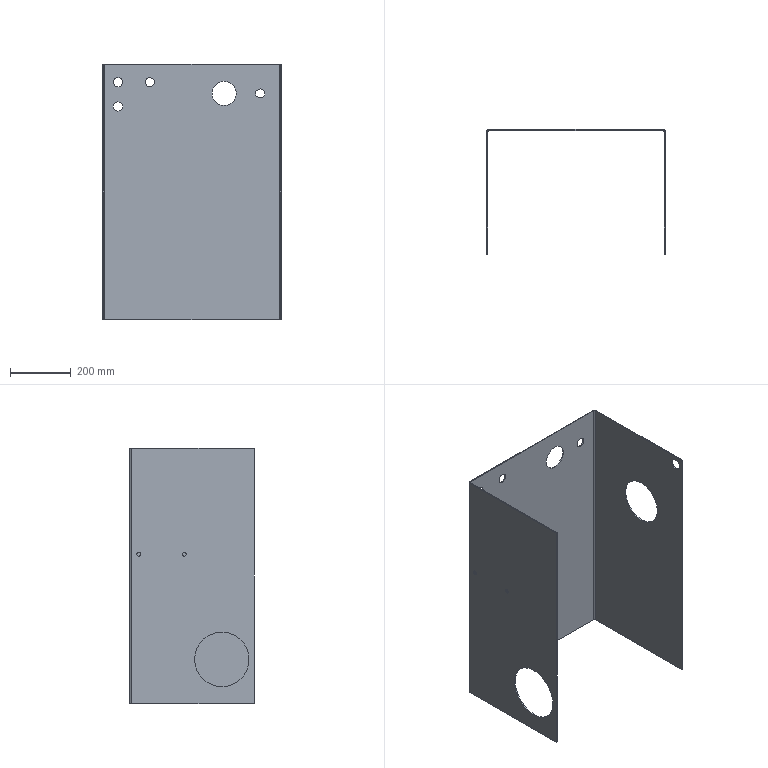Part | SolidWorks | features ICE 4, FlatPattern 1, SMBaseFlange 1, SheetMetal 1 | 1 solid | 46 faces | box 588 x 411 x 844 mm | volume 3388584 mm3 | cylinder 28 | plane 18 | commonest cylinder face diameters 30 x8 6 x6 12.5 x4 12 x2 35 x2 80 x2
STEP:
#1=CARTESIAN_POINT('',(50.,408.,689.));
#2=VERTEX_POINT('',#1);
#3=CARTESIAN_POINT('',(50.,408.,719.));
#4=VERTEX_POINT('',#3);
#5=CARTESIAN_POINT('',(50.,408.,704.));
#6=DIRECTION('',(0.,1.,0.));
#7=DIRECTION('',(0.,0.,1.));
#8=AXIS2_PLACEMENT_3D('',#5,#6,#7);
#9=CIRCLE('',#8,15.);
#10=EDGE_CURVE('',#2,#4,#9,.T.);
#11=ORIENTED_EDGE('',*,*,#10,.F.);
#12=CARTESIAN_POINT('',(50.,411.,689.));
#13=VERTEX_POINT('',#12);
#14=CARTESIAN_POINT('',(50.,401.,689.));
#15=DIRECTION('',(0.,1.,0.));
#16=VECTOR('',#15,1000.);
#17=LINE('',#14,#16);
#18=EDGE_CURVE('',#2,#13,#17,.T.);
#19=ORIENTED_EDGE('',*,*,#18,.T.);
#20=CARTESIAN_POINT('',(50.,411.,719.));
#21=VERTEX_POINT('',#20);
#22=CARTESIAN_POINT('',(50.,411.,704.));
#23=DIRECTION('',(0.,1.,0.));
#24=DIRECTION('',(0.,0.,1.));
#25=AXIS2_PLACEMENT_3D('',#22,#23,#24);
#26=CIRCLE('',#25,15.);
#27=EDGE_CURVE('',#13,#21,#26,.T.);
#28=ORIENTED_EDGE('',*,*,#27,.T.);
#29=CARTESIAN_POINT('',(50.,401.,719.));
#30=DIRECTION('',(0.,1.,0.));
#31=VECTOR('',#30,1000.);
#32=LINE('',#29,#31);
#33=EDGE_CURVE('',#4,#21,#32,.T.);
#34=ORIENTED_EDGE('',*,*,#33,.F.);
#35=EDGE_LOOP('',(#11,#19,#28,#34));
#36=FACE_OUTER_BOUND('',#35,.T.);
#37=CARTESIAN_POINT('',(50.,401.,704.));
#38=DIRECTION('',(0.,1.,0.));
#39=DIRECTION('',(0.,0.,1.));
#40=AXIS2_PLACEMENT_3D('',#37,#38,#39);
#41=CYLINDRICAL_SURFACE('',#40,15.);
#42=ADVANCED_FACE('',(#36),#41,.F.);
#43=CARTESIAN_POINT('',(50.,408.,769.));
#44=VERTEX_POINT('',#43);
#45=CARTESIAN_POINT('',(50.,408.,799.));
#46=VERTEX_POINT('',#45);
#47=CARTESIAN_POINT('',(50.,408.,784.));
#48=DIRECTION('',(0.,1.,0.));
#49=DIRECTION('',(0.,0.,1.));
#50=AXIS2_PLACEMENT_3D('',#47,#48,#49);
#51=CIRCLE('',#50,15.);
#52=EDGE_CURVE('',#44,#46,#51,.T.);
#53=ORIENTED_EDGE('',*,*,#52,.F.);
#54=CARTESIAN_POINT('',(50.,411.,769.));
#55=VERTEX_POINT('',#54);
#56=CARTESIAN_POINT('',(50.,401.,769.));
#57=DIRECTION('',(0.,1.,0.));
#58=VECTOR('',#57,1000.);
#59=LINE('',#56,#58);
#60=EDGE_CURVE('',#44,#55,#59,.T.);
#61=ORIENTED_EDGE('',*,*,#60,.T.);
#62=CARTESIAN_POINT('',(50.,411.,799.));
#63=VERTEX_POINT('',#62);
#64=CARTESIAN_POINT('',(50.,411.,784.));
#65=DIRECTION('',(0.,1.,0.));
#66=DIRECTION('',(0.,0.,1.));
#67=AXIS2_PLACEMENT_3D('',#64,#65,#66);
#68=CIRCLE('',#67,15.);
#69=EDGE_CURVE('',#55,#63,#68,.T.);
#70=ORIENTED_EDGE('',*,*,#69,.T.);
#71=CARTESIAN_POINT('',(50.,401.,799.));
#72=DIRECTION('',(0.,1.,0.));
#73=VECTOR('',#72,1000.);
#74=LINE('',#71,#73);
#75=EDGE_CURVE('',#46,#63,#74,.T.);
#76=ORIENTED_EDGE('',*,*,#75,.F.);
#77=EDGE_LOOP('',(#53,#61,#70,#76));
#78=FACE_OUTER_BOUND('',#77,.T.);
#79=CARTESIAN_POINT('',(50.,401.,784.));
#80=DIRECTION('',(0.,1.,0.));
#81=DIRECTION('',(0.,0.,1.));
#82=AXIS2_PLACEMENT_3D('',#79,#80,#81);
#83=CYLINDRICAL_SURFACE('',#82,15.);
#84=ADVANCED_FACE('',(#78),#83,.F.);
#85=CARTESIAN_POINT('',(155.,408.,769.));
#86=VERTEX_POINT('',#85);
#87=CARTESIAN_POINT('',(155.,408.,799.));
#88=VERTEX_POINT('',#87);
#89=CARTESIAN_POINT('',(155.,408.,784.));
#90=DIRECTION('',(0.,1.,0.));
#91=DIRECTION('',(0.,0.,1.));
#92=AXIS2_PLACEMENT_3D('',#89,#90,#91);
#93=CIRCLE('',#92,15.);
#94=EDGE_CURVE('',#86,#88,#93,.T.);
#95=ORIENTED_EDGE('',*,*,#94,.F.);
#96=CARTESIAN_POINT('',(155.,411.,769.));
#97=VERTEX_POINT('',#96);
#98=CARTESIAN_POINT('',(155.,401.,769.));
#99=DIRECTION('',(0.,1.,0.));
#100=VECTOR('',#99,1000.);
#101=LINE('',#98,#100);
#102=EDGE_CURVE('',#86,#97,#101,.T.);
#103=ORIENTED_EDGE('',*,*,#102,.T.);
#104=CARTESIAN_POINT('',(155.,411.,799.));
#105=VERTEX_POINT('',#104);
#106=CARTESIAN_POINT('',(155.,411.,784.));
#107=DIRECTION('',(0.,1.,0.));
#108=DIRECTION('',(0.,0.,1.));
#109=AXIS2_PLACEMENT_3D('',#106,#107,#108);
#110=CIRCLE('',#109,15.);
#111=EDGE_CURVE('',#97,#105,#110,.T.);
#112=ORIENTED_EDGE('',*,*,#111,.T.);
#113=CARTESIAN_POINT('',(155.,401.,799.));
#114=DIRECTION('',(0.,1.,0.));
#115=VECTOR('',#114,1000.);
#116=LINE('',#113,#115);
#117=EDGE_CURVE('',#88,#105,#116,.T.);
#118=ORIENTED_EDGE('',*,*,#117,.F.);
#119=EDGE_LOOP('',(#95,#103,#112,#118));
#120=FACE_OUTER_BOUND('',#119,.T.);
#121=CARTESIAN_POINT('',(155.,401.,784.));
#122=DIRECTION('',(0.,1.,0.));
#123=DIRECTION('',(0.,0.,1.));
#124=AXIS2_PLACEMENT_3D('',#121,#122,#123);
#125=CYLINDRICAL_SURFACE('',#124,15.);
#126=ADVANCED_FACE('',(#120),#125,.F.);
#127=CARTESIAN_POINT('',(519.,408.,732.));
#128=VERTEX_POINT('',#127);
#129=CARTESIAN_POINT('',(519.,408.,762.));
#130=VERTEX_POINT('',#129);
#131=CARTESIAN_POINT('',(519.,408.,747.));
#132=DIRECTION('',(0.,1.,0.));
#133=DIRECTION('',(0.,0.,1.));
#134=AXIS2_PLACEMENT_3D('',#131,#132,#133);
#135=CIRCLE('',#134,15.);
#136=EDGE_CURVE('',#128,#130,#135,.T.);
#137=ORIENTED_EDGE('',*,*,#136,.F.);
#138=CARTESIAN_POINT('',(519.,411.,732.));
#139=VERTEX_POINT('',#138);
#140=CARTESIAN_POINT('',(519.,401.,732.));
#141=DIRECTION('',(0.,1.,0.));
#142=VECTOR('',#141,1000.);
#143=LINE('',#140,#142);
#144=EDGE_CURVE('',#128,#139,#143,.T.);
#145=ORIENTED_EDGE('',*,*,#144,.T.);
#146=CARTESIAN_POINT('',(519.,411.,762.));
#147=VERTEX_POINT('',#146);
#148=CARTESIAN_POINT('',(519.,411.,747.));
#149=DIRECTION('',(0.,1.,0.));
#150=DIRECTION('',(0.,0.,1.));
#151=AXIS2_PLACEMENT_3D('',#148,#149,#150);
#152=CIRCLE('',#151,15.);
#153=EDGE_CURVE('',#139,#147,#152,.T.);
#154=ORIENTED_EDGE('',*,*,#153,.T.);
#155=CARTESIAN_POINT('',(519.,401.,762.));
#156=DIRECTION('',(0.,1.,0.));
#157=VECTOR('',#156,1000.);
#158=LINE('',#155,#157);
#159=EDGE_CURVE('',#130,#147,#158,.T.);
#160=ORIENTED_EDGE('',*,*,#159,.F.);
#161=EDGE_LOOP('',(#137,#145,#154,#160));
#162=FACE_OUTER_BOUND('',#161,.T.);
#163=CARTESIAN_POINT('',(519.,401.,747.));
#164=DIRECTION('',(0.,1.,0.));
#165=DIRECTION('',(0.,0.,1.));
#166=AXIS2_PLACEMENT_3D('',#163,#164,#165);
#167=CYLINDRICAL_SURFACE('',#166,15.);
#168=ADVANCED_FACE('',(#162),#167,.F.);
#169=CARTESIAN_POINT('',(400.,408.,707.));
#170=VERTEX_POINT('',#169);
#171=CARTESIAN_POINT('',(400.,408.,787.));
#172=VERTEX_POINT('',#171);
#173=CARTESIAN_POINT('',(400.,408.,747.));
#174=DIRECTION('',(0.,1.,0.));
#175=DIRECTION('',(0.,0.,1.));
#176=AXIS2_PLACEMENT_3D('',#173,#174,#175);
#177=CIRCLE('',#176,40.);
#178=EDGE_CURVE('',#170,#172,#177,.T.);
#179=ORIENTED_EDGE('',*,*,#178,.F.);
#180=CARTESIAN_POINT('',(400.,411.,707.));
#181=VERTEX_POINT('',#180);
#182=CARTESIAN_POINT('',(400.,401.,707.));
#183=DIRECTION('',(0.,1.,0.));
#184=VECTOR('',#183,1000.);
#185=LINE('',#182,#184);
#186=EDGE_CURVE('',#170,#181,#185,.T.);
#187=ORIENTED_EDGE('',*,*,#186,.T.);
#188=CARTESIAN_POINT('',(400.,411.,787.));
#189=VERTEX_POINT('',#188);
#190=CARTESIAN_POINT('',(400.,411.,747.));
#191=DIRECTION('',(0.,1.,0.));
#192=DIRECTION('',(0.,0.,1.));
#193=AXIS2_PLACEMENT_3D('',#190,#191,#192);
#194=CIRCLE('',#193,40.);
#195=EDGE_CURVE('',#181,#189,#194,.T.);
#196=ORIENTED_EDGE('',*,*,#195,.T.);
#197=CARTESIAN_POINT('',(400.,401.,787.));
#198=DIRECTION('',(0.,1.,0.));
#199=VECTOR('',#198,1000.);
#200=LINE('',#197,#199);
#201=EDGE_CURVE('',#172,#189,#200,.T.);
#202=ORIENTED_EDGE('',*,*,#201,.F.);
#203=EDGE_LOOP('',(#179,#187,#196,#202));
#204=FACE_OUTER_BOUND('',#203,.T.);
#205=CARTESIAN_POINT('',(400.,401.,747.));
#206=DIRECTION('',(0.,1.,0.));
#207=DIRECTION('',(0.,0.,1.));
#208=AXIS2_PLACEMENT_3D('',#205,#206,#207);
#209=CYLINDRICAL_SURFACE('',#208,40.);
#210=ADVANCED_FACE('',(#204),#209,.F.);
#211=CARTESIAN_POINT('',(585.,191.,659.));
#212=VERTEX_POINT('',#211);
#213=CARTESIAN_POINT('',(585.,191.,509.));
#214=VERTEX_POINT('',#213);
#215=CARTESIAN_POINT('',(585.,191.,584.));
#216=DIRECTION('',(1.,0.,0.));
#217=DIRECTION('',(0.,0.,-1.));
#218=AXIS2_PLACEMENT_3D('',#215,#216,#217);
#219=CIRCLE('',#218,75.);
#220=EDGE_CURVE('',#212,#214,#219,.T.);
#221=ORIENTED_EDGE('',*,*,#220,.F.);
#222=CARTESIAN_POINT('',(588.,191.,659.));
#223=VERTEX_POINT('',#222);
#224=CARTESIAN_POINT('',(578.,191.,659.));
#225=DIRECTION('',(1.,0.,0.));
#226=VECTOR('',#225,1000.);
#227=LINE('',#224,#226);
#228=EDGE_CURVE('',#212,#223,#227,.T.);
#229=ORIENTED_EDGE('',*,*,#228,.T.);
#230=CARTESIAN_POINT('',(588.,191.,509.));
#231=VERTEX_POINT('',#230);
#232=CARTESIAN_POINT('',(588.,191.,584.));
#233=DIRECTION('',(1.,0.,0.));
#234=DIRECTION('',(0.,0.,-1.));
#235=AXIS2_PLACEMENT_3D('',#232,#233,#234);
#236=CIRCLE('',#235,75.);
#237=EDGE_CURVE('',#223,#231,#236,.T.);
#238=ORIENTED_EDGE('',*,*,#237,.T.);
#239=CARTESIAN_POINT('',(578.,191.,509.));
#240=DIRECTION('',(1.,0.,0.));
#241=VECTOR('',#240,1000.);
#242=LINE('',#239,#241);
#243=EDGE_CURVE('',#214,#231,#242,.T.);
#244=ORIENTED_EDGE('',*,*,#243,.F.);
#245=EDGE_LOOP('',(#221,#229,#238,#244));
#246=FACE_OUTER_BOUND('',#245,.T.);
#247=CARTESIAN_POINT('',(578.,191.,584.));
#248=DIRECTION('',(1.,0.,0.));
#249=DIRECTION('',(0.,0.,-1.));
#250=AXIS2_PLACEMENT_3D('',#247,#248,#249);
#251=CYLINDRICAL_SURFACE('',#250,75.);
#252=ADVANCED_FACE('',(#246),#251,.F.);
#253=CARTESIAN_POINT('',(585.,30.,831.5));
#254=VERTEX_POINT('',#253);
#255=CARTESIAN_POINT('',(585.,30.,796.5));
#256=VERTEX_POINT('',#255);
#257=CARTESIAN_POINT('',(585.,30.,814.));
#258=DIRECTION('',(1.,0.,0.));
#259=DIRECTION('',(0.,0.,-1.));
#260=AXIS2_PLACEMENT_3D('',#257,#258,#259);
#261=CIRCLE('',#260,17.5);
#262=EDGE_CURVE('',#254,#256,#261,.T.);
#263=ORIENTED_EDGE('',*,*,#262,.F.);
#264=CARTESIAN_POINT('',(588.,30.,831.5));
#265=VERTEX_POINT('',#264);
#266=CARTESIAN_POINT('',(578.,30.,831.5));
#267=DIRECTION('',(1.,0.,0.));
#268=VECTOR('',#267,1000.);
#269=LINE('',#266,#268);
#270=EDGE_CURVE('',#254,#265,#269,.T.);
#271=ORIENTED_EDGE('',*,*,#270,.T.);
#272=CARTESIAN_POINT('',(588.,30.,796.5));
#273=VERTEX_POINT('',#272);
#274=CARTESIAN_POINT('',(588.,30.,814.));
#275=DIRECTION('',(1.,0.,0.));
#276=DIRECTION('',(0.,0.,-1.));
#277=AXIS2_PLACEMENT_3D('',#274,#275,#276);
#278=CIRCLE('',#277,17.5);
#279=EDGE_CURVE('',#265,#273,#278,.T.);
#280=ORIENTED_EDGE('',*,*,#279,.T.);
#281=CARTESIAN_POINT('',(578.,30.,796.5));
#282=DIRECTION('',(1.,0.,0.));
#283=VECTOR('',#282,1000.);
#284=LINE('',#281,#283);
#285=EDGE_CURVE('',#256,#273,#284,.T.);
#286=ORIENTED_EDGE('',*,*,#285,.F.);
#287=EDGE_LOOP('',(#263,#271,#280,#286));
#288=FACE_OUTER_BOUND('',#287,.T.);
#289=CARTESIAN_POINT('',(578.,30.,814.));
#290=DIRECTION('',(1.,0.,0.));
#291=DIRECTION('',(0.,0.,-1.));
#292=AXIS2_PLACEMENT_3D('',#289,#290,#291);
#293=CYLINDRICAL_SURFACE('',#292,17.5);
#294=ADVANCED_FACE('',(#288),#293,.F.);
#295=CARTESIAN_POINT('',(3.,231.,487.75));
#296=VERTEX_POINT('',#295);
#297=CARTESIAN_POINT('',(3.,231.,500.25));
#298=VERTEX_POINT('',#297);
#299=CARTESIAN_POINT('',(3.,231.,494.));
#300=DIRECTION('',(-1.,0.,0.));
#301=DIRECTION('',(0.,0.,1.));
#302=AXIS2_PLACEMENT_3D('',#299,#300,#301);
#303=CIRCLE('',#302,6.25);
#304=EDGE_CURVE('',#296,#298,#303,.T.);
#305=ORIENTED_EDGE('',*,*,#304,.F.);
#306=CARTESIAN_POINT('',(0.,231.,487.75));
#307=VERTEX_POINT('',#306);
#308=CARTESIAN_POINT('',(10.,231.,487.75));
#309=DIRECTION('',(-1.,0.,0.));
#310=VECTOR('',#309,1000.);
#311=LINE('',#308,#310);
#312=EDGE_CURVE('',#296,#307,#311,.T.);
#313=ORIENTED_EDGE('',*,*,#312,.T.);
#314=CARTESIAN_POINT('',(0.,231.,500.25));
#315=VERTEX_POINT('',#314);
#316=CARTESIAN_POINT('',(0.,231.,494.));
#317=DIRECTION('',(-1.,0.,0.));
#318=DIRECTION('',(0.,0.,1.));
#319=AXIS2_PLACEMENT_3D('',#316,#317,#318);
#320=CIRCLE('',#319,6.25);
#321=EDGE_CURVE('',#307,#315,#320,.T.);
#322=ORIENTED_EDGE('',*,*,#321,.T.);
#323=CARTESIAN_POINT('',(10.,231.,500.25));
#324=DIRECTION('',(-1.,0.,0.));
#325=VECTOR('',#324,1000.);
#326=LINE('',#323,#325);
#327=EDGE_CURVE('',#298,#315,#326,.T.);
#328=ORIENTED_EDGE('',*,*,#327,.F.);
#329=EDGE_LOOP('',(#305,#313,#322,#328));
#330=FACE_OUTER_BOUND('',#329,.T.);
#331=CARTESIAN_POINT('',(10.,231.,494.));
#332=DIRECTION('',(-1.,0.,0.));
#333=DIRECTION('',(0.,0.,1.));
#334=AXIS2_PLACEMENT_3D('',#331,#332,#333);
#335=CYLINDRICAL_SURFACE('',#334,6.25);
#336=ADVANCED_FACE('',(#330),#335,.F.);
#337=CARTESIAN_POINT('',(3.,107.,57.));
#338=VERTEX_POINT('',#337);
#339=CARTESIAN_POINT('',(3.,107.,237.));
#340=VERTEX_POINT('',#339);
#341=CARTESIAN_POINT('',(3.,107.,147.));
#342=DIRECTION('',(-1.,0.,0.));
#343=DIRECTION('',(0.,0.,1.));
#344=AXIS2_PLACEMENT_3D('',#341,#342,#343);
#345=CIRCLE('',#344,90.);
#346=EDGE_CURVE('',#338,#340,#345,.T.);
#347=ORIENTED_EDGE('',*,*,#346,.F.);
#348=CARTESIAN_POINT('',(0.,107.,57.));
#349=VERTEX_POINT('',#348);
#350=CARTESIAN_POINT('',(10.,107.,57.));
#351=DIRECTION('',(-1.,0.,0.));
#352=VECTOR('',#351,1000.);
#353=LINE('',#350,#352);
#354=EDGE_CURVE('',#338,#349,#353,.T.);
#355=ORIENTED_EDGE('',*,*,#354,.T.);
#356=CARTESIAN_POINT('',(0.,107.,237.));
#357=VERTEX_POINT('',#356);
#358=CARTESIAN_POINT('',(0.,107.,147.));
#359=DIRECTION('',(-1.,0.,0.));
#360=DIRECTION('',(0.,0.,1.));
#361=AXIS2_PLACEMENT_3D('',#358,#359,#360);
#362=CIRCLE('',#361,90.);
#363=EDGE_CURVE('',#349,#357,#362,.T.);
#364=ORIENTED_EDGE('',*,*,#363,.T.);
#365=CARTESIAN_POINT('',(10.,107.,237.));
#366=DIRECTION('',(-1.,0.,0.));
#367=VECTOR('',#366,1000.);
#368=LINE('',#365,#367);
#369=EDGE_CURVE('',#340,#357,#368,.T.);
#370=ORIENTED_EDGE('',*,*,#369,.F.);
#371=EDGE_LOOP('',(#347,#355,#364,#370));
#372=FACE_OUTER_BOUND('',#371,.T.);
#373=CARTESIAN_POINT('',(10.,107.,147.));
#374=DIRECTION('',(-1.,0.,0.));
#375=DIRECTION('',(0.,0.,1.));
#376=AXIS2_PLACEMENT_3D('',#373,#374,#375);
#377=CYLINDRICAL_SURFACE('',#376,90.);
#378=ADVANCED_FACE('',(#372),#377,.F.);
#379=CARTESIAN_POINT('',(3.,381.,487.75));
#380=VERTEX_POINT('',#379);
#381=CARTESIAN_POINT('',(3.,381.,500.25));
#382=VERTEX_POINT('',#381);
#383=CARTESIAN_POINT('',(3.,381.,494.));
#384=DIRECTION('',(-1.,0.,0.));
#385=DIRECTION('',(0.,0.,1.));
#386=AXIS2_PLACEMENT_3D('',#383,#384,#385);
#387=CIRCLE('',#386,6.25);
#388=EDGE_CURVE('',#380,#382,#387,.T.);
#389=ORIENTED_EDGE('',*,*,#388,.F.);
#390=CARTESIAN_POINT('',(0.,381.,487.75));
#391=VERTEX_POINT('',#390);
#392=CARTESIAN_POINT('',(10.,381.,487.75));
#393=DIRECTION('',(-1.,0.,0.));
#394=VECTOR('',#393,1000.);
#395=LINE('',#392,#394);
#396=EDGE_CURVE('',#380,#391,#395,.T.);
#397=ORIENTED_EDGE('',*,*,#396,.T.);
#398=CARTESIAN_POINT('',(0.,381.,500.25));
#399=VERTEX_POINT('',#398);
#400=CARTESIAN_POINT('',(0.,381.,494.));
#401=DIRECTION('',(-1.,0.,0.));
#402=DIRECTION('',(0.,0.,1.));
#403=AXIS2_PLACEMENT_3D('',#400,#401,#402);
#404=CIRCLE('',#403,6.25);
#405=EDGE_CURVE('',#391,#399,#404,.T.);
#406=ORIENTED_EDGE('',*,*,#405,.T.);
#407=CARTESIAN_POINT('',(10.,381.,500.25));
#408=DIRECTION('',(-1.,0.,0.));
#409=VECTOR('',#408,1000.);
#410=LINE('',#407,#409);
#411=EDGE_CURVE('',#382,#399,#410,.T.);
#412=ORIENTED_EDGE('',*,*,#411,.F.);
#413=EDGE_LOOP('',(#389,#397,#406,#412));
#414=FACE_OUTER_BOUND('',#413,.T.);
#415=CARTESIAN_POINT('',(10.,381.,494.));
#416=DIRECTION('',(-1.,0.,0.));
#417=DIRECTION('',(0.,0.,1.));
#418=AXIS2_PLACEMENT_3D('',#415,#416,#417);
#419=CYLINDRICAL_SURFACE('',#418,6.25);
#420=ADVANCED_FACE('',(#414),#419,.F.);
#421=CARTESIAN_POINT('',(585.,191.,584.));
#422=DIRECTION('',(1.,0.,0.));
#423=DIRECTION('',(0.,0.,-1.));
#424=AXIS2_PLACEMENT_3D('',#421,#422,#423);
#425=CIRCLE('',#424,75.);
#426=EDGE_CURVE('',#214,#212,#425,.T.);
#427=ORIENTED_EDGE('',*,*,#426,.T.);
#428=ORIENTED_EDGE('',*,*,#220,.T.);
#429=EDGE_LOOP('',(#427,#428));
#430=FACE_BOUND('',#429,.T.);
#431=CARTESIAN_POINT('',(585.,30.,814.));
#432=DIRECTION('',(1.,0.,0.));
#433=DIRECTION('',(0.,0.,-1.));
#434=AXIS2_PLACEMENT_3D('',#431,#432,#433);
#435=CIRCLE('',#434,17.5);
#436=EDGE_CURVE('',#256,#254,#435,.T.);
#437=ORIENTED_EDGE('',*,*,#436,.T.);
#438=ORIENTED_EDGE('',*,*,#262,.T.);
#439=EDGE_LOOP('',(#437,#438));
#440=FACE_BOUND('',#439,.T.);
#441=CARTESIAN_POINT('',(585.,0.,841.));
#442=VERTEX_POINT('',#441);
#443=CARTESIAN_POINT('',(585.,3.,844.));
#444=VERTEX_POINT('',#443);
#445=CARTESIAN_POINT('',(585.,3.,841.));
#446=DIRECTION('',(-1.,0.,0.));
#447=DIRECTION('',(0.,0.,-1.));
#448=AXIS2_PLACEMENT_3D('',#445,#446,#447);
#449=CIRCLE('',#448,3.);
#450=EDGE_CURVE('',#442,#444,#449,.T.);
#451=ORIENTED_EDGE('',*,*,#450,.T.);
#452=CARTESIAN_POINT('',(585.,405.,844.));
#453=VERTEX_POINT('',#452);
#454=CARTESIAN_POINT('',(585.,411.,844.));
#455=DIRECTION('',(0.,-1.,0.));
#456=VECTOR('',#455,1000.);
#457=LINE('',#454,#456);
#458=EDGE_CURVE('',#453,#444,#457,.T.);
#459=ORIENTED_EDGE('',*,*,#458,.F.);
#460=CARTESIAN_POINT('',(585.,405.,0.));
#461=VERTEX_POINT('',#460);
#462=CARTESIAN_POINT('',(585.,405.,844.));
#463=DIRECTION('',(0.,0.,-1.));
#464=VECTOR('',#463,1000.);
#465=LINE('',#462,#464);
#466=EDGE_CURVE('',#453,#461,#465,.T.);
#467=ORIENTED_EDGE('',*,*,#466,.T.);
#468=CARTESIAN_POINT('',(585.,3.,0.));
#469=VERTEX_POINT('',#468);
#470=CARTESIAN_POINT('',(585.,411.,0.));
#471=DIRECTION('',(0.,-1.,0.));
#472=VECTOR('',#471,1000.);
#473=LINE('',#470,#472);
#474=EDGE_CURVE('',#461,#469,#473,.T.);
#475=ORIENTED_EDGE('',*,*,#474,.T.);
#476=CARTESIAN_POINT('',(585.,0.,3.));
#477=VERTEX_POINT('',#476);
#478=CARTESIAN_POINT('',(585.,3.,3.));
#479=DIRECTION('',(-1.,0.,0.));
#480=DIRECTION('',(0.,0.,-1.));
#481=AXIS2_PLACEMENT_3D('',#478,#479,#480);
#482=CIRCLE('',#481,3.);
#483=EDGE_CURVE('',#469,#477,#482,.T.);
#484=ORIENTED_EDGE('',*,*,#483,.T.);
#485=CARTESIAN_POINT('',(585.,0.,844.));
#486=DIRECTION('',(0.,0.,-1.));
#487=VECTOR('',#486,1000.);
#488=LINE('',#485,#487);
#489=EDGE_CURVE('',#442,#477,#488,.T.);
#490=ORIENTED_EDGE('',*,*,#489,.F.);
#491=EDGE_LOOP('',(#451,#459,#467,#475,#484,#490));
#492=FACE_OUTER_BOUND('',#491,.T.);
#493=CARTESIAN_POINT('',(585.,411.,844.));
#494=DIRECTION('',(1.,0.,0.));
#495=DIRECTION('',(0.,0.,-1.));
#496=AXIS2_PLACEMENT_3D('',#493,#494,#495);
#497=PLANE('',#496);
#498=ADVANCED_FACE('',(#430,#440,#492),#497,.F.);
#499=CARTESIAN_POINT('',(588.,191.,584.));
#500=DIRECTION('',(1.,0.,0.));
#501=DIRECTION('',(0.,0.,-1.));
#502=AXIS2_PLACEMENT_3D('',#499,#500,#501);
#503=CIRCLE('',#502,75.);
#504=EDGE_CURVE('',#231,#223,#503,.T.);
#505=ORIENTED_EDGE('',*,*,#504,.F.);
#506=ORIENTED_EDGE('',*,*,#237,.F.);
#507=EDGE_LOOP('',(#505,#506));
#508=FACE_BOUND('',#507,.T.);
#509=CARTESIAN_POINT('',(588.,30.,814.));
#510=DIRECTION('',(1.,0.,0.));
#511=DIRECTION('',(0.,0.,-1.));
#512=AXIS2_PLACEMENT_3D('',#509,#510,#511);
#513=CIRCLE('',#512,17.5);
#514=EDGE_CURVE('',#273,#265,#513,.T.);
#515=ORIENTED_EDGE('',*,*,#514,.F.);
#516=ORIENTED_EDGE('',*,*,#279,.F.);
#517=EDGE_LOOP('',(#515,#516));
#518=FACE_BOUND('',#517,.T.);
#519=CARTESIAN_POINT('',(588.,405.,844.));
#520=VERTEX_POINT('',#519);
#521=CARTESIAN_POINT('',(588.,3.,844.));
#522=VERTEX_POINT('',#521);
#523=CARTESIAN_POINT('',(588.,411.,844.));
#524=DIRECTION('',(0.,-1.,0.));
#525=VECTOR('',#524,1000.);
#526=LINE('',#523,#525);
#527=EDGE_CURVE('',#520,#522,#526,.T.);
#528=ORIENTED_EDGE('',*,*,#527,.T.);
#529=CARTESIAN_POINT('',(588.,0.,841.));
#530=VERTEX_POINT('',#529);
#531=CARTESIAN_POINT('',(588.,3.,841.));
#532=DIRECTION('',(-1.,0.,0.));
#533=DIRECTION('',(0.,0.,-1.));
#534=AXIS2_PLACEMENT_3D('',#531,#532,#533);
#535=CIRCLE('',#534,3.);
#536=EDGE_CURVE('',#530,#522,#535,.T.);
#537=ORIENTED_EDGE('',*,*,#536,.F.);
#538=CARTESIAN_POINT('',(588.,0.,3.));
#539=VERTEX_POINT('',#538);
#540=CARTESIAN_POINT('',(588.,0.,844.));
#541=DIRECTION('',(0.,0.,-1.));
#542=VECTOR('',#541,1000.);
#543=LINE('',#540,#542);
#544=EDGE_CURVE('',#530,#539,#543,.T.);
#545=ORIENTED_EDGE('',*,*,#544,.T.);
#546=CARTESIAN_POINT('',(588.,3.,0.));
#547=VERTEX_POINT('',#546);
#548=CARTESIAN_POINT('',(588.,3.,3.));
#549=DIRECTION('',(-1.,0.,0.));
#550=DIRECTION('',(0.,0.,-1.));
#551=AXIS2_PLACEMENT_3D('',#548,#549,#550);
#552=CIRCLE('',#551,3.);
#553=EDGE_CURVE('',#547,#539,#552,.T.);
#554=ORIENTED_EDGE('',*,*,#553,.F.);
#555=CARTESIAN_POINT('',(588.,405.,0.));
#556=VERTEX_POINT('',#555);
#557=CARTESIAN_POINT('',(588.,411.,0.));
#558=DIRECTION('',(0.,-1.,0.));
#559=VECTOR('',#558,1000.);
#560=LINE('',#557,#559);
#561=EDGE_CURVE('',#556,#547,#560,.T.);
#562=ORIENTED_EDGE('',*,*,#561,.F.);
#563=CARTESIAN_POINT('',(588.,405.,844.));
#564=DIRECTION('',(0.,0.,-1.));
#565=VECTOR('',#564,1000.);
#566=LINE('',#563,#565);
#567=EDGE_CURVE('',#520,#556,#566,.T.);
#568=ORIENTED_EDGE('',*,*,#567,.F.);
#569=EDGE_LOOP('',(#528,#537,#545,#554,#562,#568));
#570=FACE_OUTER_BOUND('',#569,.T.);
#571=CARTESIAN_POINT('',(588.,411.,844.));
#572=DIRECTION('',(1.,0.,0.));
#573=DIRECTION('',(0.,0.,-1.));
#574=AXIS2_PLACEMENT_3D('',#571,#572,#573);
#575=PLANE('',#574);
#576=ADVANCED_FACE('',(#508,#518,#570),#575,.T.);
#577=ORIENTED_EDGE('',*,*,#458,.T.);
#578=CARTESIAN_POINT('',(585.,3.,844.));
#579=DIRECTION('',(1.,0.,0.));
#580=VECTOR('',#579,1000.);
#581=LINE('',#578,#580);
#582=EDGE_CURVE('',#444,#522,#581,.T.);
#583=ORIENTED_EDGE('',*,*,#582,.T.);
#584=ORIENTED_EDGE('',*,*,#527,.F.);
#585=CARTESIAN_POINT('',(588.,405.,844.));
#586=DIRECTION('',(-1.,0.,0.));
#587=VECTOR('',#586,1000.);
#588=LINE('',#585,#587);
#589=EDGE_CURVE('',#520,#453,#588,.T.);
#590=ORIENTED_EDGE('',*,*,#589,.T.);
#591=EDGE_LOOP('',(#577,#583,#584,#590));
#592=FACE_OUTER_BOUND('',#591,.T.);
#593=CARTESIAN_POINT('',(582.,408.,844.));
#594=DIRECTION('',(0.,0.,1.));
#595=DIRECTION('',(1.,0.,0.));
#596=AXIS2_PLACEMENT_3D('',#593,#594,#595);
#597=PLANE('',#596);
#598=ADVANCED_FACE('',(#592),#597,.T.);
#599=CARTESIAN_POINT('',(585.,0.,841.));
#600=DIRECTION('',(1.,0.,0.));
#601=VECTOR('',#600,1000.);
#602=LINE('',#599,#601);
#603=EDGE_CURVE('',#442,#530,#602,.T.);
#604=ORIENTED_EDGE('',*,*,#603,.F.);
#605=ORIENTED_EDGE('',*,*,#489,.T.);
#606=CARTESIAN_POINT('',(585.,0.,3.));
#607=DIRECTION('',(1.,0.,0.));
#608=VECTOR('',#607,1000.);
#609=LINE('',#606,#608);
#610=EDGE_CURVE('',#477,#539,#609,.T.);
#611=ORIENTED_EDGE('',*,*,#610,.T.);
#612=ORIENTED_EDGE('',*,*,#544,.F.);
#613=EDGE_LOOP('',(#604,#605,#611,#612));
#614=FACE_OUTER_BOUND('',#613,.T.);
#615=CARTESIAN_POINT('',(588.,0.,844.));
#616=DIRECTION('',(0.,-1.,0.));
#617=DIRECTION('',(0.,0.,-1.));
#618=AXIS2_PLACEMENT_3D('',#615,#616,#617);
#619=PLANE('',#618);
#620=ADVANCED_FACE('',(#614),#619,.T.);
#621=CARTESIAN_POINT('',(585.,3.,0.));
#622=DIRECTION('',(1.,0.,0.));
#623=VECTOR('',#622,1000.);
#624=LINE('',#621,#623);
#625=EDGE_CURVE('',#469,#547,#624,.T.);
#626=ORIENTED_EDGE('',*,*,#625,.F.);
#627=ORIENTED_EDGE('',*,*,#474,.F.);
#628=CARTESIAN_POINT('',(585.,405.,0.));
#629=DIRECTION('',(1.,0.,0.));
#630=VECTOR('',#629,1000.);
#631=LINE('',#628,#630);
#632=EDGE_CURVE('',#461,#556,#631,.T.);
#633=ORIENTED_EDGE('',*,*,#632,.T.);
#634=ORIENTED_EDGE('',*,*,#561,.T.);
#635=EDGE_LOOP('',(#626,#627,#633,#634));
#636=FACE_OUTER_BOUND('',#635,.T.);
#637=CARTESIAN_POINT('',(582.,405.,0.));
#638=DIRECTION('',(0.,0.,1.));
#639=DIRECTION('',(1.,0.,0.));
#640=AXIS2_PLACEMENT_3D('',#637,#638,#639);
#641=PLANE('',#640);
#642=ADVANCED_FACE('',(#636),#641,.F.);
#643=CARTESIAN_POINT('',(0.,231.,494.));
#644=DIRECTION('',(-1.,0.,0.));
#645=DIRECTION('',(0.,0.,1.));
#646=AXIS2_PLACEMENT_3D('',#643,#644,#645);
#647=CIRCLE('',#646,6.25);
#648=EDGE_CURVE('',#315,#307,#647,.T.);
#649=ORIENTED_EDGE('',*,*,#648,.F.);
#650=ORIENTED_EDGE('',*,*,#321,.F.);
#651=EDGE_LOOP('',(#649,#650));
#652=FACE_BOUND('',#651,.T.);
#653=CARTESIAN_POINT('',(0.,107.,147.));
#654=DIRECTION('',(-1.,0.,0.));
#655=DIRECTION('',(0.,0.,1.));
#656=AXIS2_PLACEMENT_3D('',#653,#654,#655);
#657=CIRCLE('',#656,90.);
#658=EDGE_CURVE('',#357,#349,#657,.T.);
#659=ORIENTED_EDGE('',*,*,#658,.F.);
#660=ORIENTED_EDGE('',*,*,#363,.F.);
#661=EDGE_LOOP('',(#659,#660));
#662=FACE_BOUND('',#661,.T.);
#663=CARTESIAN_POINT('',(0.,381.,494.));
#664=DIRECTION('',(-1.,0.,0.));
#665=DIRECTION('',(0.,0.,1.));
#666=AXIS2_PLACEMENT_3D('',#663,#664,#665);
#667=CIRCLE('',#666,6.25);
#668=EDGE_CURVE('',#399,#391,#667,.T.);
#669=ORIENTED_EDGE('',*,*,#668,.F.);
#670=ORIENTED_EDGE('',*,*,#405,.F.);
#671=EDGE_LOOP('',(#669,#670));
#672=FACE_BOUND('',#671,.T.);
#673=CARTESIAN_POINT('',(0.,0.,841.));
#674=VERTEX_POINT('',#673);
#675=CARTESIAN_POINT('',(0.,0.,3.));
#676=VERTEX_POINT('',#675);
#677=CARTESIAN_POINT('',(0.,0.,844.));
#678=DIRECTION('',(0.,0.,-1.));
#679=VECTOR('',#678,1000.);
#680=LINE('',#677,#679);
#681=EDGE_CURVE('',#674,#676,#680,.T.);
#682=ORIENTED_EDGE('',*,*,#681,.F.);
#683=CARTESIAN_POINT('',(0.,3.,844.));
#684=VERTEX_POINT('',#683);
#685=CARTESIAN_POINT('',(0.,3.,841.));
#686=DIRECTION('',(1.,0.,0.));
#687=DIRECTION('',(0.,0.,1.));
#688=AXIS2_PLACEMENT_3D('',#685,#686,#687);
#689=CIRCLE('',#688,3.);
#690=EDGE_CURVE('',#684,#674,#689,.T.);
#691=ORIENTED_EDGE('',*,*,#690,.F.);
#692=CARTESIAN_POINT('',(0.,405.,844.));
#693=VERTEX_POINT('',#692);
#694=CARTESIAN_POINT('',(0.,0.,844.));
#695=DIRECTION('',(0.,1.,0.));
#696=VECTOR('',#695,1000.);
#697=LINE('',#694,#696);
#698=EDGE_CURVE('',#684,#693,#697,.T.);
#699=ORIENTED_EDGE('',*,*,#698,.T.);
#700=CARTESIAN_POINT('',(0.,405.,0.));
#701=VERTEX_POINT('',#700);
#702=CARTESIAN_POINT('',(0.,405.,844.));
#703=DIRECTION('',(0.,0.,-1.));
#704=VECTOR('',#703,1000.);
#705=LINE('',#702,#704);
#706=EDGE_CURVE('',#693,#701,#705,.T.);
#707=ORIENTED_EDGE('',*,*,#706,.T.);
#708=CARTESIAN_POINT('',(0.,3.,0.));
#709=VERTEX_POINT('',#708);
#710=CARTESIAN_POINT('',(0.,0.,0.));
#711=DIRECTION('',(0.,1.,0.));
#712=VECTOR('',#711,1000.);
#713=LINE('',#710,#712);
#714=EDGE_CURVE('',#709,#701,#713,.T.);
#715=ORIENTED_EDGE('',*,*,#714,.F.);
#716=CARTESIAN_POINT('',(0.,3.,3.));
#717=DIRECTION('',(1.,0.,0.));
#718=DIRECTION('',(0.,0.,1.));
#719=AXIS2_PLACEMENT_3D('',#716,#717,#718);
#720=CIRCLE('',#719,3.);
#721=EDGE_CURVE('',#676,#709,#720,.T.);
#722=ORIENTED_EDGE('',*,*,#721,.F.);
#723=EDGE_LOOP('',(#682,#691,#699,#707,#715,#722));
#724=FACE_OUTER_BOUND('',#723,.T.);
#725=CARTESIAN_POINT('',(0.,0.,844.));
#726=DIRECTION('',(-1.,0.,0.));
#727=DIRECTION('',(0.,0.,1.));
#728=AXIS2_PLACEMENT_3D('',#725,#726,#727);
#729=PLANE('',#728);
#730=ADVANCED_FACE('',(#652,#662,#672,#724),#729,.T.);
#731=CARTESIAN_POINT('',(3.,231.,494.));
#732=DIRECTION('',(-1.,0.,0.));
#733=DIRECTION('',(0.,0.,1.));
#734=AXIS2_PLACEMENT_3D('',#731,#732,#733);
#735=CIRCLE('',#734,6.25);
#736=EDGE_CURVE('',#298,#296,#735,.T.);
#737=ORIENTED_EDGE('',*,*,#736,.T.);
#738=ORIENTED_EDGE('',*,*,#304,.T.);
#739=EDGE_LOOP('',(#737,#738));
#740=FACE_BOUND('',#739,.T.);
#741=CARTESIAN_POINT('',(3.,107.,147.));
#742=DIRECTION('',(-1.,0.,0.));
#743=DIRECTION('',(0.,0.,1.));
#744=AXIS2_PLACEMENT_3D('',#741,#742,#743);
#745=CIRCLE('',#744,90.);
#746=EDGE_CURVE('',#340,#338,#745,.T.);
#747=ORIENTED_EDGE('',*,*,#746,.T.);
#748=ORIENTED_EDGE('',*,*,#346,.T.);
#749=EDGE_LOOP('',(#747,#748));
#750=FACE_BOUND('',#749,.T.);
#751=CARTESIAN_POINT('',(3.,381.,494.));
#752=DIRECTION('',(-1.,0.,0.));
#753=DIRECTION('',(0.,0.,1.));
#754=AXIS2_PLACEMENT_3D('',#751,#752,#753);
#755=CIRCLE('',#754,6.25);
#756=EDGE_CURVE('',#382,#380,#755,.T.);
#757=ORIENTED_EDGE('',*,*,#756,.T.);
#758=ORIENTED_EDGE('',*,*,#388,.T.);
#759=EDGE_LOOP('',(#757,#758));
#760=FACE_BOUND('',#759,.T.);
#761=CARTESIAN_POINT('',(3.,3.,844.));
#762=VERTEX_POINT('',#761);
#763=CARTESIAN_POINT('',(3.,0.,841.));
#764=VERTEX_POINT('',#763);
#765=CARTESIAN_POINT('',(3.,3.,841.));
#766=DIRECTION('',(1.,0.,0.));
#767=DIRECTION('',(0.,0.,1.));
#768=AXIS2_PLACEMENT_3D('',#765,#766,#767);
#769=CIRCLE('',#768,3.);
#770=EDGE_CURVE('',#762,#764,#769,.T.);
#771=ORIENTED_EDGE('',*,*,#770,.T.);
#772=CARTESIAN_POINT('',(3.,0.,3.));
#773=VERTEX_POINT('',#772);
#774=CARTESIAN_POINT('',(3.,0.,844.));
#775=DIRECTION('',(0.,0.,-1.));
#776=VECTOR('',#775,1000.);
#777=LINE('',#774,#776);
#778=EDGE_CURVE('',#764,#773,#777,.T.);
#779=ORIENTED_EDGE('',*,*,#778,.T.);
#780=CARTESIAN_POINT('',(3.,3.,0.));
#781=VERTEX_POINT('',#780);
#782=CARTESIAN_POINT('',(3.,3.,3.));
#783=DIRECTION('',(1.,0.,0.));
#784=DIRECTION('',(0.,0.,1.));
#785=AXIS2_PLACEMENT_3D('',#782,#783,#784);
#786=CIRCLE('',#785,3.);
#787=EDGE_CURVE('',#773,#781,#786,.T.);
#788=ORIENTED_EDGE('',*,*,#787,.T.);
#789=CARTESIAN_POINT('',(3.,405.,0.));
#790=VERTEX_POINT('',#789);
#791=CARTESIAN_POINT('',(3.,0.,0.));
#792=DIRECTION('',(0.,1.,0.));
#793=VECTOR('',#792,1000.);
#794=LINE('',#791,#793);
#795=EDGE_CURVE('',#781,#790,#794,.T.);
#796=ORIENTED_EDGE('',*,*,#795,.T.);
#797=CARTESIAN_POINT('',(3.,405.,844.));
#798=VERTEX_POINT('',#797);
#799=CARTESIAN_POINT('',(3.,405.,844.));
#800=DIRECTION('',(0.,0.,-1.));
#801=VECTOR('',#800,1000.);
#802=LINE('',#799,#801);
#803=EDGE_CURVE('',#798,#790,#802,.T.);
#804=ORIENTED_EDGE('',*,*,#803,.F.);
#805=CARTESIAN_POINT('',(3.,0.,844.));
#806=DIRECTION('',(0.,1.,0.));
#807=VECTOR('',#806,1000.);
#808=LINE('',#805,#807);
#809=EDGE_CURVE('',#762,#798,#808,.T.);
#810=ORIENTED_EDGE('',*,*,#809,.F.);
#811=EDGE_LOOP('',(#771,#779,#788,#796,#804,#810));
#812=FACE_OUTER_BOUND('',#811,.T.);
#813=CARTESIAN_POINT('',(3.,0.,844.));
#814=DIRECTION('',(-1.,0.,0.));
#815=DIRECTION('',(0.,0.,1.));
#816=AXIS2_PLACEMENT_3D('',#813,#814,#815);
#817=PLANE('',#816);
#818=ADVANCED_FACE('',(#740,#750,#760,#812),#817,.F.);
#819=ORIENTED_EDGE('',*,*,#778,.F.);
#820=CARTESIAN_POINT('',(3.,0.,841.));
#821=DIRECTION('',(-1.,0.,0.));
#822=VECTOR('',#821,1000.);
#823=LINE('',#820,#822);
#824=EDGE_CURVE('',#764,#674,#823,.T.);
#825=ORIENTED_EDGE('',*,*,#824,.T.);
#826=ORIENTED_EDGE('',*,*,#681,.T.);
#827=CARTESIAN_POINT('',(3.,0.,3.));
#828=DIRECTION('',(-1.,0.,0.));
#829=VECTOR('',#828,1000.);
#830=LINE('',#827,#829);
#831=EDGE_CURVE('',#773,#676,#830,.T.);
#832=ORIENTED_EDGE('',*,*,#831,.F.);
#833=EDGE_LOOP('',(#819,#825,#826,#832));
#834=FACE_OUTER_BOUND('',#833,.T.);
#835=CARTESIAN_POINT('',(3.,0.,844.));
#836=DIRECTION('',(0.,-1.,0.));
#837=DIRECTION('',(0.,0.,-1.));
#838=AXIS2_PLACEMENT_3D('',#835,#836,#837);
#839=PLANE('',#838);
#840=ADVANCED_FACE('',(#834),#839,.T.);
#841=ORIENTED_EDGE('',*,*,#795,.F.);
#842=CARTESIAN_POINT('',(3.,3.,0.));
#843=DIRECTION('',(-1.,0.,0.));
#844=VECTOR('',#843,1000.);
#845=LINE('',#842,#844);
#846=EDGE_CURVE('',#781,#709,#845,.T.);
#847=ORIENTED_EDGE('',*,*,#846,.T.);
#848=ORIENTED_EDGE('',*,*,#714,.T.);
#849=CARTESIAN_POINT('',(0.,405.,0.));
#850=DIRECTION('',(1.,0.,0.));
#851=VECTOR('',#850,1000.);
#852=LINE('',#849,#851);
#853=EDGE_CURVE('',#701,#790,#852,.T.);
#854=ORIENTED_EDGE('',*,*,#853,.T.);
#855=EDGE_LOOP('',(#841,#847,#848,#854));
#856=FACE_OUTER_BOUND('',#855,.T.);
#857=CARTESIAN_POINT('',(6.,408.,0.));
#858=DIRECTION('',(0.,0.,-1.));
#859=DIRECTION('',(-1.,0.,0.));
#860=AXIS2_PLACEMENT_3D('',#857,#858,#859);
#861=PLANE('',#860);
#862=ADVANCED_FACE('',(#856),#861,.T.);
#863=CARTESIAN_POINT('',(6.,411.,844.));
#864=VERTEX_POINT('',#863);
#865=CARTESIAN_POINT('',(6.,408.,844.));
#866=VERTEX_POINT('',#865);
#867=CARTESIAN_POINT('',(6.,411.,844.));
#868=DIRECTION('',(0.,-1.,0.));
#869=VECTOR('',#868,1000.);
#870=LINE('',#867,#869);
#871=EDGE_CURVE('',#864,#866,#870,.T.);
#872=ORIENTED_EDGE('',*,*,#871,.F.);
#873=CARTESIAN_POINT('',(6.,405.,844.));
#874=DIRECTION('',(0.,0.,-1.));
#875=DIRECTION('',(1.,0.,0.));
#876=AXIS2_PLACEMENT_3D('',#873,#874,#875);
#877=CIRCLE('',#876,6.);
#878=EDGE_CURVE('',#693,#864,#877,.T.);
#879=ORIENTED_EDGE('',*,*,#878,.F.);
#880=CARTESIAN_POINT('',(3.,405.,844.));
#881=DIRECTION('',(-1.,0.,0.));
#882=VECTOR('',#881,1000.);
#883=LINE('',#880,#882);
#884=EDGE_CURVE('',#798,#693,#883,.T.);
#885=ORIENTED_EDGE('',*,*,#884,.F.);
#886=CARTESIAN_POINT('',(6.,405.,844.));
#887=DIRECTION('',(0.,0.,-1.));
#888=DIRECTION('',(1.,0.,0.));
#889=AXIS2_PLACEMENT_3D('',#886,#887,#888);
#890=CIRCLE('',#889,3.);
#891=EDGE_CURVE('',#798,#866,#890,.T.);
#892=ORIENTED_EDGE('',*,*,#891,.T.);
#893=EDGE_LOOP('',(#872,#879,#885,#892));
#894=FACE_OUTER_BOUND('',#893,.T.);
#895=CARTESIAN_POINT('',(6.,411.,844.));
#896=DIRECTION('',(0.,0.,1.));
#897=DIRECTION('',(1.,0.,0.));
#898=AXIS2_PLACEMENT_3D('',#895,#896,#897);
#899=PLANE('',#898);
#900=ADVANCED_FACE('',(#894),#899,.T.);
#901=CARTESIAN_POINT('',(582.,411.,844.));
#902=VERTEX_POINT('',#901);
#903=CARTESIAN_POINT('',(0.,411.,844.));
#904=DIRECTION('',(1.,0.,0.));
#905=VECTOR('',#904,1000.);
#906=LINE('',#903,#905);
#907=EDGE_CURVE('',#864,#902,#906,.T.);
#908=ORIENTED_EDGE('',*,*,#907,.F.);
#909=ORIENTED_EDGE('',*,*,#871,.T.);
#910=CARTESIAN_POINT('',(582.,408.,844.));
#911=VERTEX_POINT('',#910);
#912=CARTESIAN_POINT('',(0.,408.,844.));
#913=DIRECTION('',(1.,0.,0.));
#914=VECTOR('',#913,1000.);
#915=LINE('',#912,#914);
#916=EDGE_CURVE('',#866,#911,#915,.T.);
#917=ORIENTED_EDGE('',*,*,#916,.T.);
#918=CARTESIAN_POINT('',(582.,408.,844.));
#919=DIRECTION('',(0.,1.,0.));
#920=VECTOR('',#919,1000.);
#921=LINE('',#918,#920);
#922=EDGE_CURVE('',#911,#902,#921,.T.);
#923=ORIENTED_EDGE('',*,*,#922,.T.);
#924=EDGE_LOOP('',(#908,#909,#917,#923));
#925=FACE_OUTER_BOUND('',#924,.T.);
#926=CARTESIAN_POINT('',(3.,405.,844.));
#927=DIRECTION('',(0.,0.,1.));
#928=DIRECTION('',(1.,0.,0.));
#929=AXIS2_PLACEMENT_3D('',#926,#927,#928);
#930=PLANE('',#929);
#931=ADVANCED_FACE('',(#925),#930,.T.);
#932=ORIENTED_EDGE('',*,*,#853,.F.);
#933=CARTESIAN_POINT('',(6.,411.,0.));
#934=VERTEX_POINT('',#933);
#935=CARTESIAN_POINT('',(6.,405.,0.));
#936=DIRECTION('',(0.,0.,-1.));
#937=DIRECTION('',(1.,0.,0.));
#938=AXIS2_PLACEMENT_3D('',#935,#936,#937);
#939=CIRCLE('',#938,6.);
#940=EDGE_CURVE('',#701,#934,#939,.T.);
#941=ORIENTED_EDGE('',*,*,#940,.T.);
#942=CARTESIAN_POINT('',(6.,408.,0.));
#943=VERTEX_POINT('',#942);
#944=CARTESIAN_POINT('',(6.,408.,0.));
#945=DIRECTION('',(0.,1.,0.));
#946=VECTOR('',#945,1000.);
#947=LINE('',#944,#946);
#948=EDGE_CURVE('',#943,#934,#947,.T.);
#949=ORIENTED_EDGE('',*,*,#948,.F.);
#950=CARTESIAN_POINT('',(6.,405.,0.));
#951=DIRECTION('',(0.,0.,-1.));
#952=DIRECTION('',(1.,0.,0.));
#953=AXIS2_PLACEMENT_3D('',#950,#951,#952);
#954=CIRCLE('',#953,3.);
#955=EDGE_CURVE('',#790,#943,#954,.T.);
#956=ORIENTED_EDGE('',*,*,#955,.F.);
#957=EDGE_LOOP('',(#932,#941,#949,#956));
#958=FACE_OUTER_BOUND('',#957,.T.);
#959=CARTESIAN_POINT('',(0.,405.,0.));
#960=DIRECTION('',(0.,0.,-1.));
#961=DIRECTION('',(-1.,0.,0.));
#962=AXIS2_PLACEMENT_3D('',#959,#960,#961);
#963=PLANE('',#962);
#964=ADVANCED_FACE('',(#958),#963,.T.);
#965=ORIENTED_EDGE('',*,*,#589,.F.);
#966=CARTESIAN_POINT('',(582.,405.,844.));
#967=DIRECTION('',(0.,0.,-1.));
#968=DIRECTION('',(1.,0.,0.));
#969=AXIS2_PLACEMENT_3D('',#966,#967,#968);
#970=CIRCLE('',#969,6.);
#971=EDGE_CURVE('',#902,#520,#970,.T.);
#972=ORIENTED_EDGE('',*,*,#971,.F.);
#973=ORIENTED_EDGE('',*,*,#922,.F.);
#974=CARTESIAN_POINT('',(582.,405.,844.));
#975=DIRECTION('',(0.,0.,-1.));
#976=DIRECTION('',(1.,0.,0.));
#977=AXIS2_PLACEMENT_3D('',#974,#975,#976);
#978=CIRCLE('',#977,3.);
#979=EDGE_CURVE('',#911,#453,#978,.T.);
#980=ORIENTED_EDGE('',*,*,#979,.T.);
#981=EDGE_LOOP('',(#965,#972,#973,#980));
#982=FACE_OUTER_BOUND('',#981,.T.);
#983=CARTESIAN_POINT('',(588.,405.,844.));
#984=DIRECTION('',(0.,0.,1.));
#985=DIRECTION('',(1.,0.,0.));
#986=AXIS2_PLACEMENT_3D('',#983,#984,#985);
#987=PLANE('',#986);
#988=ADVANCED_FACE('',(#982),#987,.T.);
#989=CARTESIAN_POINT('',(582.,411.,0.));
#990=VERTEX_POINT('',#989);
#991=CARTESIAN_POINT('',(582.,408.,0.));
#992=VERTEX_POINT('',#991);
#993=CARTESIAN_POINT('',(582.,411.,0.));
#994=DIRECTION('',(0.,-1.,0.));
#995=VECTOR('',#994,1000.);
#996=LINE('',#993,#995);
#997=EDGE_CURVE('',#990,#992,#996,.T.);
#998=ORIENTED_EDGE('',*,*,#997,.F.);
#999=CARTESIAN_POINT('',(582.,405.,0.));
#1000=DIRECTION('',(0.,0.,-1.));
#1001=DIRECTION('',(1.,0.,0.));
#1002=AXIS2_PLACEMENT_3D('',#999,#1000,#1001);
#1003=CIRCLE('',#1002,6.);
#1004=EDGE_CURVE('',#990,#556,#1003,.T.);
#1005=ORIENTED_EDGE('',*,*,#1004,.T.);
#1006=ORIENTED_EDGE('',*,*,#632,.F.);
#1007=CARTESIAN_POINT('',(582.,405.,0.));
#1008=DIRECTION('',(0.,0.,-1.));
#1009=DIRECTION('',(1.,0.,0.));
#1010=AXIS2_PLACEMENT_3D('',#1007,#1008,#1009);
#1011=CIRCLE('',#1010,3.);
#1012=EDGE_CURVE('',#992,#461,#1011,.T.);
#1013=ORIENTED_EDGE('',*,*,#1012,.F.);
#1014=EDGE_LOOP('',(#998,#1005,#1006,#1013));
#1015=FACE_OUTER_BOUND('',#1014,.T.);
#1016=CARTESIAN_POINT('',(582.,411.,0.));
#1017=DIRECTION('',(0.,0.,-1.));
#1018=DIRECTION('',(-1.,0.,0.));
#1019=AXIS2_PLACEMENT_3D('',#1016,#1017,#1018);
#1020=PLANE('',#1019);
#1021=ADVANCED_FACE('',(#1015),#1020,.T.);
#1022=CARTESIAN_POINT('',(0.,411.,0.));
#1023=DIRECTION('',(1.,0.,0.));
#1024=VECTOR('',#1023,1000.);
#1025=LINE('',#1022,#1024);
#1026=EDGE_CURVE('',#934,#990,#1025,.T.);
#1027=ORIENTED_EDGE('',*,*,#1026,.T.);
#1028=ORIENTED_EDGE('',*,*,#997,.T.);
#1029=CARTESIAN_POINT('',(0.,408.,0.));
#1030=DIRECTION('',(1.,0.,0.));
#1031=VECTOR('',#1030,1000.);
#1032=LINE('',#1029,#1031);
#1033=EDGE_CURVE('',#943,#992,#1032,.T.);
#1034=ORIENTED_EDGE('',*,*,#1033,.F.);
#1035=ORIENTED_EDGE('',*,*,#948,.T.);
#1036=EDGE_LOOP('',(#1027,#1028,#1034,#1035));
#1037=FACE_OUTER_BOUND('',#1036,.T.);
#1038=CARTESIAN_POINT('',(585.,405.,0.));
#1039=DIRECTION('',(0.,0.,-1.));
#1040=DIRECTION('',(-1.,0.,0.));
#1041=AXIS2_PLACEMENT_3D('',#1038,#1039,#1040);
#1042=PLANE('',#1041);
#1043=ADVANCED_FACE('',(#1037),#1042,.T.);
#1044=ORIENTED_EDGE('',*,*,#1004,.F.);
#1045=CARTESIAN_POINT('',(582.,411.,844.));
#1046=DIRECTION('',(0.,0.,-1.));
#1047=VECTOR('',#1046,1000.);
#1048=LINE('',#1045,#1047);
#1049=EDGE_CURVE('',#902,#990,#1048,.T.);
#1050=ORIENTED_EDGE('',*,*,#1049,.F.);
#1051=ORIENTED_EDGE('',*,*,#971,.T.);
#1052=ORIENTED_EDGE('',*,*,#567,.T.);
#1053=EDGE_LOOP('',(#1044,#1050,#1051,#1052));
#1054=FACE_OUTER_BOUND('',#1053,.T.);
#1055=CARTESIAN_POINT('',(582.,405.,844.));
#1056=DIRECTION('',(0.,0.,-1.));
#1057=DIRECTION('',(-1.,0.,0.));
#1058=AXIS2_PLACEMENT_3D('',#1055,#1056,#1057);
#1059=CYLINDRICAL_SURFACE('',#1058,6.);
#1060=ADVANCED_FACE('',(#1054),#1059,.T.);
#1061=CARTESIAN_POINT('',(50.,411.,704.));
#1062=DIRECTION('',(0.,1.,0.));
#1063=DIRECTION('',(0.,0.,1.));
#1064=AXIS2_PLACEMENT_3D('',#1061,#1062,#1063);
#1065=CIRCLE('',#1064,15.);
#1066=EDGE_CURVE('',#21,#13,#1065,.T.);
#1067=ORIENTED_EDGE('',*,*,#1066,.F.);
#1068=ORIENTED_EDGE('',*,*,#27,.F.);
#1069=EDGE_LOOP('',(#1067,#1068));
#1070=FACE_BOUND('',#1069,.T.);
#1071=CARTESIAN_POINT('',(50.,411.,784.));
#1072=DIRECTION('',(0.,1.,0.));
#1073=DIRECTION('',(0.,0.,1.));
#1074=AXIS2_PLACEMENT_3D('',#1071,#1072,#1073);
#1075=CIRCLE('',#1074,15.);
#1076=EDGE_CURVE('',#63,#55,#1075,.T.);
#1077=ORIENTED_EDGE('',*,*,#1076,.F.);
#1078=ORIENTED_EDGE('',*,*,#69,.F.);
#1079=EDGE_LOOP('',(#1077,#1078));
#1080=FACE_BOUND('',#1079,.T.);
#1081=CARTESIAN_POINT('',(155.,411.,784.));
#1082=DIRECTION('',(0.,1.,0.));
#1083=DIRECTION('',(0.,0.,1.));
#1084=AXIS2_PLACEMENT_3D('',#1081,#1082,#1083);
#1085=CIRCLE('',#1084,15.);
#1086=EDGE_CURVE('',#105,#97,#1085,.T.);
#1087=ORIENTED_EDGE('',*,*,#1086,.F.);
#1088=ORIENTED_EDGE('',*,*,#111,.F.);
#1089=EDGE_LOOP('',(#1087,#1088));
#1090=FACE_BOUND('',#1089,.T.);
#1091=CARTESIAN_POINT('',(519.,411.,747.));
#1092=DIRECTION('',(0.,1.,0.));
#1093=DIRECTION('',(0.,0.,1.));
#1094=AXIS2_PLACEMENT_3D('',#1091,#1092,#1093);
#1095=CIRCLE('',#1094,15.);
#1096=EDGE_CURVE('',#147,#139,#1095,.T.);
#1097=ORIENTED_EDGE('',*,*,#1096,.F.);
#1098=ORIENTED_EDGE('',*,*,#153,.F.);
#1099=EDGE_LOOP('',(#1097,#1098));
#1100=FACE_BOUND('',#1099,.T.);
#1101=CARTESIAN_POINT('',(400.,411.,747.));
#1102=DIRECTION('',(0.,1.,0.));
#1103=DIRECTION('',(0.,0.,1.));
#1104=AXIS2_PLACEMENT_3D('',#1101,#1102,#1103);
#1105=CIRCLE('',#1104,40.);
#1106=EDGE_CURVE('',#189,#181,#1105,.T.);
#1107=ORIENTED_EDGE('',*,*,#1106,.F.);
#1108=ORIENTED_EDGE('',*,*,#195,.F.);
#1109=EDGE_LOOP('',(#1107,#1108));
#1110=FACE_BOUND('',#1109,.T.);
#1111=ORIENTED_EDGE('',*,*,#1026,.F.);
#1112=CARTESIAN_POINT('',(6.,411.,844.));
#1113=DIRECTION('',(0.,0.,-1.));
#1114=VECTOR('',#1113,1000.);
#1115=LINE('',#1112,#1114);
#1116=EDGE_CURVE('',#864,#934,#1115,.T.);
#1117=ORIENTED_EDGE('',*,*,#1116,.F.);
#1118=ORIENTED_EDGE('',*,*,#907,.T.);
#1119=ORIENTED_EDGE('',*,*,#1049,.T.);
#1120=EDGE_LOOP('',(#1111,#1117,#1118,#1119));
#1121=FACE_OUTER_BOUND('',#1120,.T.);
#1122=CARTESIAN_POINT('',(0.,411.,844.));
#1123=DIRECTION('',(0.,1.,0.));
#1124=DIRECTION('',(0.,0.,1.));
#1125=AXIS2_PLACEMENT_3D('',#1122,#1123,#1124);
#1126=PLANE('',#1125);
#1127=ADVANCED_FACE('',(#1070,#1080,#1090,#1100,#1110,#1121),#1126,.T.);
#1128=ORIENTED_EDGE('',*,*,#940,.F.);
#1129=ORIENTED_EDGE('',*,*,#706,.F.);
#1130=ORIENTED_EDGE('',*,*,#878,.T.);
#1131=ORIENTED_EDGE('',*,*,#1116,.T.);
#1132=EDGE_LOOP('',(#1128,#1129,#1130,#1131));
#1133=FACE_OUTER_BOUND('',#1132,.T.);
#1134=CARTESIAN_POINT('',(6.,405.,844.));
#1135=DIRECTION('',(0.,0.,-1.));
#1136=DIRECTION('',(-1.,0.,0.));
#1137=AXIS2_PLACEMENT_3D('',#1134,#1135,#1136);
#1138=CYLINDRICAL_SURFACE('',#1137,6.);
#1139=ADVANCED_FACE('',(#1133),#1138,.T.);
#1140=ORIENTED_EDGE('',*,*,#955,.T.);
#1141=CARTESIAN_POINT('',(6.,408.,844.));
#1142=DIRECTION('',(0.,0.,-1.));
#1143=VECTOR('',#1142,1000.);
#1144=LINE('',#1141,#1143);
#1145=EDGE_CURVE('',#866,#943,#1144,.T.);
#1146=ORIENTED_EDGE('',*,*,#1145,.F.);
#1147=ORIENTED_EDGE('',*,*,#891,.F.);
#1148=ORIENTED_EDGE('',*,*,#803,.T.);
#1149=EDGE_LOOP('',(#1140,#1146,#1147,#1148));
#1150=FACE_OUTER_BOUND('',#1149,.T.);
#1151=CARTESIAN_POINT('',(6.,405.,844.));
#1152=DIRECTION('',(0.,0.,-1.));
#1153=DIRECTION('',(-1.,0.,0.));
#1154=AXIS2_PLACEMENT_3D('',#1151,#1152,#1153);
#1155=CYLINDRICAL_SURFACE('',#1154,3.);
#1156=ADVANCED_FACE('',(#1150),#1155,.F.);
#1157=CARTESIAN_POINT('',(50.,408.,704.));
#1158=DIRECTION('',(0.,1.,0.));
#1159=DIRECTION('',(0.,0.,1.));
#1160=AXIS2_PLACEMENT_3D('',#1157,#1158,#1159);
#1161=CIRCLE('',#1160,15.);
#1162=EDGE_CURVE('',#4,#2,#1161,.T.);
#1163=ORIENTED_EDGE('',*,*,#1162,.T.);
#1164=ORIENTED_EDGE('',*,*,#10,.T.);
#1165=EDGE_LOOP('',(#1163,#1164));
#1166=FACE_BOUND('',#1165,.T.);
#1167=CARTESIAN_POINT('',(50.,408.,784.));
#1168=DIRECTION('',(0.,1.,0.));
#1169=DIRECTION('',(0.,0.,1.));
#1170=AXIS2_PLACEMENT_3D('',#1167,#1168,#1169);
#1171=CIRCLE('',#1170,15.);
#1172=EDGE_CURVE('',#46,#44,#1171,.T.);
#1173=ORIENTED_EDGE('',*,*,#1172,.T.);
#1174=ORIENTED_EDGE('',*,*,#52,.T.);
#1175=EDGE_LOOP('',(#1173,#1174));
#1176=FACE_BOUND('',#1175,.T.);
#1177=CARTESIAN_POINT('',(155.,408.,784.));
#1178=DIRECTION('',(0.,1.,0.));
#1179=DIRECTION('',(0.,0.,1.));
#1180=AXIS2_PLACEMENT_3D('',#1177,#1178,#1179);
#1181=CIRCLE('',#1180,15.);
#1182=EDGE_CURVE('',#88,#86,#1181,.T.);
#1183=ORIENTED_EDGE('',*,*,#1182,.T.);
#1184=ORIENTED_EDGE('',*,*,#94,.T.);
#1185=EDGE_LOOP('',(#1183,#1184));
#1186=FACE_BOUND('',#1185,.T.);
#1187=CARTESIAN_POINT('',(519.,408.,747.));
#1188=DIRECTION('',(0.,1.,0.));
#1189=DIRECTION('',(0.,0.,1.));
#1190=AXIS2_PLACEMENT_3D('',#1187,#1188,#1189);
#1191=CIRCLE('',#1190,15.);
#1192=EDGE_CURVE('',#130,#128,#1191,.T.);
#1193=ORIENTED_EDGE('',*,*,#1192,.T.);
#1194=ORIENTED_EDGE('',*,*,#136,.T.);
#1195=EDGE_LOOP('',(#1193,#1194));
#1196=FACE_BOUND('',#1195,.T.);
#1197=CARTESIAN_POINT('',(400.,408.,747.));
#1198=DIRECTION('',(0.,1.,0.));
#1199=DIRECTION('',(0.,0.,1.));
#1200=AXIS2_PLACEMENT_3D('',#1197,#1198,#1199);
#1201=CIRCLE('',#1200,40.);
#1202=EDGE_CURVE('',#172,#170,#1201,.T.);
#1203=ORIENTED_EDGE('',*,*,#1202,.T.);
#1204=ORIENTED_EDGE('',*,*,#178,.T.);
#1205=EDGE_LOOP('',(#1203,#1204));
#1206=FACE_BOUND('',#1205,.T.);
#1207=ORIENTED_EDGE('',*,*,#1033,.T.);
#1208=CARTESIAN_POINT('',(582.,408.,844.));
#1209=DIRECTION('',(0.,0.,-1.));
#1210=VECTOR('',#1209,1000.);
#1211=LINE('',#1208,#1210);
#1212=EDGE_CURVE('',#911,#992,#1211,.T.);
#1213=ORIENTED_EDGE('',*,*,#1212,.F.);
#1214=ORIENTED_EDGE('',*,*,#916,.F.);
#1215=ORIENTED_EDGE('',*,*,#1145,.T.);
#1216=EDGE_LOOP('',(#1207,#1213,#1214,#1215));
#1217=FACE_OUTER_BOUND('',#1216,.T.);
#1218=CARTESIAN_POINT('',(0.,408.,844.));
#1219=DIRECTION('',(0.,1.,0.));
#1220=DIRECTION('',(0.,0.,1.));
#1221=AXIS2_PLACEMENT_3D('',#1218,#1219,#1220);
#1222=PLANE('',#1221);
#1223=ADVANCED_FACE('',(#1166,#1176,#1186,#1196,#1206,#1217),#1222,.F.);
#1224=ORIENTED_EDGE('',*,*,#1012,.T.);
#1225=ORIENTED_EDGE('',*,*,#466,.F.);
#1226=ORIENTED_EDGE('',*,*,#979,.F.);
#1227=ORIENTED_EDGE('',*,*,#1212,.T.);
#1228=EDGE_LOOP('',(#1224,#1225,#1226,#1227));
#1229=FACE_OUTER_BOUND('',#1228,.T.);
#1230=CARTESIAN_POINT('',(582.,405.,844.));
#1231=DIRECTION('',(0.,0.,-1.));
#1232=DIRECTION('',(-1.,0.,0.));
#1233=AXIS2_PLACEMENT_3D('',#1230,#1231,#1232);
#1234=CYLINDRICAL_SURFACE('',#1233,3.);
#1235=ADVANCED_FACE('',(#1229),#1234,.F.);
#1236=CARTESIAN_POINT('',(3.,3.,844.));
#1237=DIRECTION('',(-1.,0.,0.));
#1238=VECTOR('',#1237,1000.);
#1239=LINE('',#1236,#1238);
#1240=EDGE_CURVE('',#762,#684,#1239,.T.);
#1241=ORIENTED_EDGE('',*,*,#1240,.F.);
#1242=ORIENTED_EDGE('',*,*,#809,.T.);
#1243=ORIENTED_EDGE('',*,*,#884,.T.);
#1244=ORIENTED_EDGE('',*,*,#698,.F.);
#1245=EDGE_LOOP('',(#1241,#1242,#1243,#1244));
#1246=FACE_OUTER_BOUND('',#1245,.T.);
#1247=CARTESIAN_POINT('',(582.,405.,844.));
#1248=DIRECTION('',(0.,0.,1.));
#1249=DIRECTION('',(1.,0.,0.));
#1250=AXIS2_PLACEMENT_3D('',#1247,#1248,#1249);
#1251=PLANE('',#1250);
#1252=ADVANCED_FACE('',(#1246),#1251,.T.);
#1253=ORIENTED_EDGE('',*,*,#396,.F.);
#1254=ORIENTED_EDGE('',*,*,#756,.F.);
#1255=ORIENTED_EDGE('',*,*,#411,.T.);
#1256=ORIENTED_EDGE('',*,*,#668,.T.);
#1257=EDGE_LOOP('',(#1253,#1254,#1255,#1256));
#1258=FACE_OUTER_BOUND('',#1257,.T.);
#1259=CARTESIAN_POINT('',(10.,381.,494.));
#1260=DIRECTION('',(-1.,0.,0.));
#1261=DIRECTION('',(0.,0.,1.));
#1262=AXIS2_PLACEMENT_3D('',#1259,#1260,#1261);
#1263=CYLINDRICAL_SURFACE('',#1262,6.25);
#1264=ADVANCED_FACE('',(#1258),#1263,.F.);
#1265=ORIENTED_EDGE('',*,*,#354,.F.);
#1266=ORIENTED_EDGE('',*,*,#746,.F.);
#1267=ORIENTED_EDGE('',*,*,#369,.T.);
#1268=ORIENTED_EDGE('',*,*,#658,.T.);
#1269=EDGE_LOOP('',(#1265,#1266,#1267,#1268));
#1270=FACE_OUTER_BOUND('',#1269,.T.);
#1271=CARTESIAN_POINT('',(10.,107.,147.));
#1272=DIRECTION('',(-1.,0.,0.));
#1273=DIRECTION('',(0.,0.,1.));
#1274=AXIS2_PLACEMENT_3D('',#1271,#1272,#1273);
#1275=CYLINDRICAL_SURFACE('',#1274,90.);
#1276=ADVANCED_FACE('',(#1270),#1275,.F.);
#1277=ORIENTED_EDGE('',*,*,#312,.F.);
#1278=ORIENTED_EDGE('',*,*,#736,.F.);
#1279=ORIENTED_EDGE('',*,*,#327,.T.);
#1280=ORIENTED_EDGE('',*,*,#648,.T.);
#1281=EDGE_LOOP('',(#1277,#1278,#1279,#1280));
#1282=FACE_OUTER_BOUND('',#1281,.T.);
#1283=CARTESIAN_POINT('',(10.,231.,494.));
#1284=DIRECTION('',(-1.,0.,0.));
#1285=DIRECTION('',(0.,0.,1.));
#1286=AXIS2_PLACEMENT_3D('',#1283,#1284,#1285);
#1287=CYLINDRICAL_SURFACE('',#1286,6.25);
#1288=ADVANCED_FACE('',(#1282),#1287,.F.);
#1289=ORIENTED_EDGE('',*,*,#270,.F.);
#1290=ORIENTED_EDGE('',*,*,#436,.F.);
#1291=ORIENTED_EDGE('',*,*,#285,.T.);
#1292=ORIENTED_EDGE('',*,*,#514,.T.);
#1293=EDGE_LOOP('',(#1289,#1290,#1291,#1292));
#1294=FACE_OUTER_BOUND('',#1293,.T.);
#1295=CARTESIAN_POINT('',(578.,30.,814.));
#1296=DIRECTION('',(1.,0.,0.));
#1297=DIRECTION('',(0.,0.,-1.));
#1298=AXIS2_PLACEMENT_3D('',#1295,#1296,#1297);
#1299=CYLINDRICAL_SURFACE('',#1298,17.5);
#1300=ADVANCED_FACE('',(#1294),#1299,.F.);
#1301=ORIENTED_EDGE('',*,*,#228,.F.);
#1302=ORIENTED_EDGE('',*,*,#426,.F.);
#1303=ORIENTED_EDGE('',*,*,#243,.T.);
#1304=ORIENTED_EDGE('',*,*,#504,.T.);
#1305=EDGE_LOOP('',(#1301,#1302,#1303,#1304));
#1306=FACE_OUTER_BOUND('',#1305,.T.);
#1307=CARTESIAN_POINT('',(578.,191.,584.));
#1308=DIRECTION('',(1.,0.,0.));
#1309=DIRECTION('',(0.,0.,-1.));
#1310=AXIS2_PLACEMENT_3D('',#1307,#1308,#1309);
#1311=CYLINDRICAL_SURFACE('',#1310,75.);
#1312=ADVANCED_FACE('',(#1306),#1311,.F.);
#1313=ORIENTED_EDGE('',*,*,#186,.F.);
#1314=ORIENTED_EDGE('',*,*,#1202,.F.);
#1315=ORIENTED_EDGE('',*,*,#201,.T.);
#1316=ORIENTED_EDGE('',*,*,#1106,.T.);
#1317=EDGE_LOOP('',(#1313,#1314,#1315,#1316));
#1318=FACE_OUTER_BOUND('',#1317,.T.);
#1319=CARTESIAN_POINT('',(400.,401.,747.));
#1320=DIRECTION('',(0.,1.,0.));
#1321=DIRECTION('',(0.,0.,1.));
#1322=AXIS2_PLACEMENT_3D('',#1319,#1320,#1321);
#1323=CYLINDRICAL_SURFACE('',#1322,40.);
#1324=ADVANCED_FACE('',(#1318),#1323,.F.);
#1325=ORIENTED_EDGE('',*,*,#144,.F.);
#1326=ORIENTED_EDGE('',*,*,#1192,.F.);
#1327=ORIENTED_EDGE('',*,*,#159,.T.);
#1328=ORIENTED_EDGE('',*,*,#1096,.T.);
#1329=EDGE_LOOP('',(#1325,#1326,#1327,#1328));
#1330=FACE_OUTER_BOUND('',#1329,.T.);
#1331=CARTESIAN_POINT('',(519.,401.,747.));
#1332=DIRECTION('',(0.,1.,0.));
#1333=DIRECTION('',(0.,0.,1.));
#1334=AXIS2_PLACEMENT_3D('',#1331,#1332,#1333);
#1335=CYLINDRICAL_SURFACE('',#1334,15.);
#1336=ADVANCED_FACE('',(#1330),#1335,.F.);
#1337=ORIENTED_EDGE('',*,*,#102,.F.);
#1338=ORIENTED_EDGE('',*,*,#1182,.F.);
#1339=ORIENTED_EDGE('',*,*,#117,.T.);
#1340=ORIENTED_EDGE('',*,*,#1086,.T.);
#1341=EDGE_LOOP('',(#1337,#1338,#1339,#1340));
#1342=FACE_OUTER_BOUND('',#1341,.T.);
#1343=CARTESIAN_POINT('',(155.,401.,784.));
#1344=DIRECTION('',(0.,1.,0.));
#1345=DIRECTION('',(0.,0.,1.));
#1346=AXIS2_PLACEMENT_3D('',#1343,#1344,#1345);
#1347=CYLINDRICAL_SURFACE('',#1346,15.);
#1348=ADVANCED_FACE('',(#1342),#1347,.F.);
#1349=ORIENTED_EDGE('',*,*,#60,.F.);
#1350=ORIENTED_EDGE('',*,*,#1172,.F.);
#1351=ORIENTED_EDGE('',*,*,#75,.T.);
#1352=ORIENTED_EDGE('',*,*,#1076,.T.);
#1353=EDGE_LOOP('',(#1349,#1350,#1351,#1352));
#1354=FACE_OUTER_BOUND('',#1353,.T.);
#1355=CARTESIAN_POINT('',(50.,401.,784.));
#1356=DIRECTION('',(0.,1.,0.));
#1357=DIRECTION('',(0.,0.,1.));
#1358=AXIS2_PLACEMENT_3D('',#1355,#1356,#1357);
#1359=CYLINDRICAL_SURFACE('',#1358,15.);
#1360=ADVANCED_FACE('',(#1354),#1359,.F.);
#1361=ORIENTED_EDGE('',*,*,#18,.F.);
#1362=ORIENTED_EDGE('',*,*,#1162,.F.);
#1363=ORIENTED_EDGE('',*,*,#33,.T.);
#1364=ORIENTED_EDGE('',*,*,#1066,.T.);
#1365=EDGE_LOOP('',(#1361,#1362,#1363,#1364));
#1366=FACE_OUTER_BOUND('',#1365,.T.);
#1367=CARTESIAN_POINT('',(50.,401.,704.));
#1368=DIRECTION('',(0.,1.,0.));
#1369=DIRECTION('',(0.,0.,1.));
#1370=AXIS2_PLACEMENT_3D('',#1367,#1368,#1369);
#1371=CYLINDRICAL_SURFACE('',#1370,15.);
#1372=ADVANCED_FACE('',(#1366),#1371,.F.);
#1373=ORIENTED_EDGE('',*,*,#846,.F.);
#1374=ORIENTED_EDGE('',*,*,#787,.F.);
#1375=ORIENTED_EDGE('',*,*,#831,.T.);
#1376=ORIENTED_EDGE('',*,*,#721,.T.);
#1377=EDGE_LOOP('',(#1373,#1374,#1375,#1376));
#1378=FACE_OUTER_BOUND('',#1377,.T.);
#1379=CARTESIAN_POINT('',(3.,3.,3.));
#1380=DIRECTION('',(-1.,0.,0.));
#1381=DIRECTION('',(0.,0.,1.));
#1382=AXIS2_PLACEMENT_3D('',#1379,#1380,#1381);
#1383=CYLINDRICAL_SURFACE('',#1382,3.);
#1384=ADVANCED_FACE('',(#1378),#1383,.T.);
#1385=ORIENTED_EDGE('',*,*,#824,.F.);
#1386=ORIENTED_EDGE('',*,*,#770,.F.);
#1387=ORIENTED_EDGE('',*,*,#1240,.T.);
#1388=ORIENTED_EDGE('',*,*,#690,.T.);
#1389=EDGE_LOOP('',(#1385,#1386,#1387,#1388));
#1390=FACE_OUTER_BOUND('',#1389,.T.);
#1391=CARTESIAN_POINT('',(3.,3.,841.));
#1392=DIRECTION('',(-1.,0.,0.));
#1393=DIRECTION('',(0.,0.,1.));
#1394=AXIS2_PLACEMENT_3D('',#1391,#1392,#1393);
#1395=CYLINDRICAL_SURFACE('',#1394,3.);
#1396=ADVANCED_FACE('',(#1390),#1395,.T.);
#1397=ORIENTED_EDGE('',*,*,#610,.F.);
#1398=ORIENTED_EDGE('',*,*,#483,.F.);
#1399=ORIENTED_EDGE('',*,*,#625,.T.);
#1400=ORIENTED_EDGE('',*,*,#553,.T.);
#1401=EDGE_LOOP('',(#1397,#1398,#1399,#1400));
#1402=FACE_OUTER_BOUND('',#1401,.T.);
#1403=CARTESIAN_POINT('',(585.,3.,3.));
#1404=DIRECTION('',(1.,0.,0.));
#1405=DIRECTION('',(0.,0.,-1.));
#1406=AXIS2_PLACEMENT_3D('',#1403,#1404,#1405);
#1407=CYLINDRICAL_SURFACE('',#1406,3.);
#1408=ADVANCED_FACE('',(#1402),#1407,.T.);
#1409=ORIENTED_EDGE('',*,*,#582,.F.);
#1410=ORIENTED_EDGE('',*,*,#450,.F.);
#1411=ORIENTED_EDGE('',*,*,#603,.T.);
#1412=ORIENTED_EDGE('',*,*,#536,.T.);
#1413=EDGE_LOOP('',(#1409,#1410,#1411,#1412));
#1414=FACE_OUTER_BOUND('',#1413,.T.);
#1415=CARTESIAN_POINT('',(585.,3.,841.));
#1416=DIRECTION('',(1.,0.,0.));
#1417=DIRECTION('',(0.,0.,-1.));
#1418=AXIS2_PLACEMENT_3D('',#1415,#1416,#1417);
#1419=CYLINDRICAL_SURFACE('',#1418,3.);
#1420=ADVANCED_FACE('',(#1414),#1419,.T.);
#1421=CLOSED_SHELL('',(#42,#84,#126,#168,#210,#252,#294,#336,#378,#420,#498,#576,#598,#620,#642,#730,#818,#840,#862,#900,#931,#964,#988,#1021,#1043,#1060,#1127,#1139,#1156,#1223,#1235,#1252,#1264,#1276,#1288,#1300,#1312,#1324,#1336,#1348,#1360,#1372,#1384,#1396,#1408,#1420));
#1422=MANIFOLD_SOLID_BREP('',#1421);
#1423=CARTESIAN_POINT('',(0.,0.,0.));
#1424=DIRECTION('',(0.,0.,1.));
#1425=DIRECTION('',(1.,0.,0.));
#1426=AXIS2_PLACEMENT_3D('',#1423,#1424,#1425);
#1427=(LENGTH_UNIT()NAMED_UNIT(*)SI_UNIT(.MILLI.,.METRE.));
#1428=UNCERTAINTY_MEASURE_WITH_UNIT(LENGTH_MEASURE(0.00001),#1427,'','');
#1429=(NAMED_UNIT(*)PLANE_ANGLE_UNIT()SI_UNIT($,.RADIAN.));
#1430=(NAMED_UNIT(*)SI_UNIT($,.STERADIAN.)SOLID_ANGLE_UNIT());
#1431=(GEOMETRIC_REPRESENTATION_CONTEXT(3)GLOBAL_UNCERTAINTY_ASSIGNED_CONTEXT((#1428))GLOBAL_UNIT_ASSIGNED_CONTEXT((#1427,#1429,#1430))REPRESENTATION_CONTEXT('',''));
#1432=ADVANCED_BREP_SHAPE_REPRESENTATION('',(#1422,#1426),#1431);